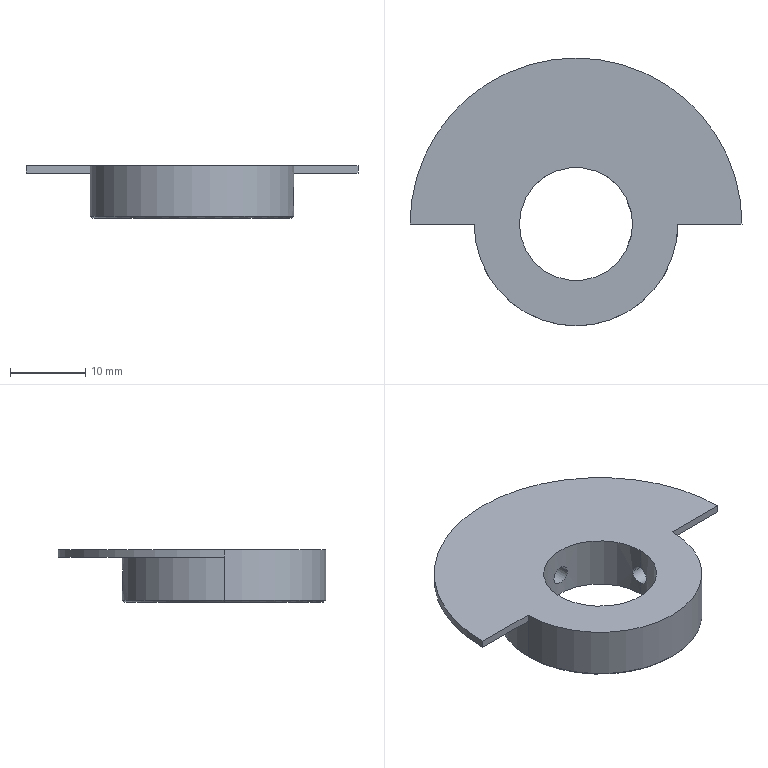Part | NX | 1 solid | 20 faces | box 44 x 35.5 x 7 mm | volume 3181 mm3 | cylinder 9 | plane 5 | spline 4 | cone 2 | commonest cylinder face diameters 2.5 x4 15 x2 27 x2 44 x1
STEP:
#1=CARTESIAN_POINT('',(13.2,0.,-7.));
#2=VERTEX_POINT('',#1);
#3=CARTESIAN_POINT('',(-13.2,0.,-7.));
#4=VERTEX_POINT('',#3);
#5=CARTESIAN_POINT('',(0.,0.,-7.));
#6=DIRECTION('',(0.,0.,-1.));
#7=DIRECTION('',(1.,0.,0.));
#8=AXIS2_PLACEMENT_3D('',#5,#6,#7);
#9=CIRCLE('',#8,13.2);
#10=EDGE_CURVE('',#2,#4,#9,.T.);
#11=ORIENTED_EDGE('',*,*,#10,.T.);
#12=CARTESIAN_POINT('',(0.,0.,-7.));
#13=DIRECTION('',(0.,0.,-1.));
#14=DIRECTION('',(1.,0.,0.));
#15=AXIS2_PLACEMENT_3D('',#12,#13,#14);
#16=CIRCLE('',#15,13.2);
#17=EDGE_CURVE('',#4,#2,#16,.T.);
#18=ORIENTED_EDGE('',*,*,#17,.T.);
#19=EDGE_LOOP('',(#11,#18));
#20=FACE_BOUND('',#19,.T.);
#21=CARTESIAN_POINT('',(7.5,0.,-7.));
#22=VERTEX_POINT('',#21);
#23=CARTESIAN_POINT('',(-7.5,0.,-7.));
#24=VERTEX_POINT('',#23);
#25=CARTESIAN_POINT('',(0.,0.,-7.));
#26=DIRECTION('',(0.,0.,1.));
#27=DIRECTION('',(1.,0.,0.));
#28=AXIS2_PLACEMENT_3D('',#25,#26,#27);
#29=CIRCLE('',#28,7.5);
#30=EDGE_CURVE('',#22,#24,#29,.T.);
#31=ORIENTED_EDGE('',*,*,#30,.T.);
#32=CARTESIAN_POINT('',(0.,0.,-7.));
#33=DIRECTION('',(0.,0.,1.));
#34=DIRECTION('',(1.,0.,0.));
#35=AXIS2_PLACEMENT_3D('',#32,#33,#34);
#36=CIRCLE('',#35,7.5);
#37=EDGE_CURVE('',#24,#22,#36,.T.);
#38=ORIENTED_EDGE('',*,*,#37,.T.);
#39=EDGE_LOOP('',(#31,#38));
#40=FACE_BOUND('',#39,.T.);
#41=CARTESIAN_POINT('',(0.,0.,-7.));
#42=DIRECTION('',(0.,0.,1.));
#43=DIRECTION('',(1.,0.,0.));
#44=AXIS2_PLACEMENT_3D('',#41,#42,#43);
#45=PLANE('',#44);
#46=ADVANCED_FACE('',(#20,#40),#45,.F.);
#47=CARTESIAN_POINT('',(-13.5,0.,0.));
#48=VERTEX_POINT('',#47);
#49=CARTESIAN_POINT('',(-13.5,0.,-1.));
#50=VERTEX_POINT('',#49);
#51=CARTESIAN_POINT('',(-13.5,0.,0.));
#52=DIRECTION('',(0.,0.,-1.));
#53=VECTOR('',#52,1000.);
#54=LINE('',#51,#53);
#55=EDGE_CURVE('',#48,#50,#54,.T.);
#56=ORIENTED_EDGE('',*,*,#55,.T.);
#57=CARTESIAN_POINT('',(-13.5,0.,-6.7));
#58=VERTEX_POINT('',#57);
#59=CARTESIAN_POINT('',(-13.5,0.,0.));
#60=DIRECTION('',(0.,0.,-1.));
#61=VECTOR('',#60,1000.);
#62=LINE('',#59,#61);
#63=EDGE_CURVE('',#58,#50,#62,.F.);
#64=ORIENTED_EDGE('',*,*,#63,.F.);
#65=CARTESIAN_POINT('',(13.5,0.,-6.7));
#66=VERTEX_POINT('',#65);
#67=CARTESIAN_POINT('',(0.,0.,-6.7));
#68=DIRECTION('',(0.,0.,-1.));
#69=DIRECTION('',(1.,0.,0.));
#70=AXIS2_PLACEMENT_3D('',#67,#68,#69);
#71=CIRCLE('',#70,13.5);
#72=EDGE_CURVE('',#66,#58,#71,.T.);
#73=ORIENTED_EDGE('',*,*,#72,.F.);
#74=CARTESIAN_POINT('',(13.5,0.,-5.7));
#75=VERTEX_POINT('',#74);
#76=CARTESIAN_POINT('',(13.5,0.,0.));
#77=DIRECTION('',(0.,0.,-1.));
#78=VECTOR('',#77,1000.);
#79=LINE('',#76,#78);
#80=EDGE_CURVE('',#75,#66,#79,.T.);
#81=ORIENTED_EDGE('',*,*,#80,.F.);
#82=CARTESIAN_POINT('',(13.5,-0.01096,-5.7));
#83=VERTEX_POINT('',#82);
#84=CARTESIAN_POINT('',(13.5,0.,-5.7));
#85=CARTESIAN_POINT('',(13.5,-0.003653,-5.7));
#86=CARTESIAN_POINT('',(13.5,-0.007306,-5.7));
#87=CARTESIAN_POINT('',(13.5,-0.01096,-5.7));
#88=B_SPLINE_CURVE_WITH_KNOTS('',3,(#84,#85,#86,#87),.UNSPECIFIED.,.F.,.F.,(4,4),(0.,1.),.UNSPECIFIED.);
#89=EDGE_CURVE('',#75,#83,#88,.T.);
#90=ORIENTED_EDGE('',*,*,#89,.T.);
#91=CARTESIAN_POINT('',(13.5,0.,-2.3));
#92=VERTEX_POINT('',#91);
#93=CARTESIAN_POINT('',(13.5,-0.01096,-5.7));
#94=CARTESIAN_POINT('',(13.499,-0.9006,-5.694));
#95=CARTESIAN_POINT('',(13.303,-2.364,-3.994));
#96=CARTESIAN_POINT('',(13.5,-0.8891,-2.3));
#97=CARTESIAN_POINT('',(13.5,0.,-2.3));
#98=B_SPLINE_CURVE_WITH_KNOTS('',3,(#93,#94,#95,#96,#97),.UNSPECIFIED.,.F.,.F.,(4,1,4),(0.,0.5,1.),.UNSPECIFIED.);
#99=EDGE_CURVE('',#83,#92,#98,.T.);
#100=ORIENTED_EDGE('',*,*,#99,.T.);
#101=CARTESIAN_POINT('',(13.5,0.,-1.));
#102=VERTEX_POINT('',#101);
#103=CARTESIAN_POINT('',(13.5,0.,0.));
#104=DIRECTION('',(0.,0.,-1.));
#105=VECTOR('',#104,1000.);
#106=LINE('',#103,#105);
#107=EDGE_CURVE('',#92,#102,#106,.F.);
#108=ORIENTED_EDGE('',*,*,#107,.T.);
#109=CARTESIAN_POINT('',(13.5,0.,0.));
#110=VERTEX_POINT('',#109);
#111=CARTESIAN_POINT('',(13.5,0.,0.));
#112=DIRECTION('',(0.,0.,-1.));
#113=VECTOR('',#112,1000.);
#114=LINE('',#111,#113);
#115=EDGE_CURVE('',#110,#102,#114,.T.);
#116=ORIENTED_EDGE('',*,*,#115,.F.);
#117=CARTESIAN_POINT('',(0.,0.,0.));
#118=DIRECTION('',(0.,0.,1.));
#119=DIRECTION('',(-1.,0.,0.));
#120=AXIS2_PLACEMENT_3D('',#117,#118,#119);
#121=CIRCLE('',#120,13.5);
#122=EDGE_CURVE('',#48,#110,#121,.T.);
#123=ORIENTED_EDGE('',*,*,#122,.F.);
#124=EDGE_LOOP('',(#56,#64,#73,#81,#90,#100,#108,#116,#123));
#125=FACE_BOUND('',#124,.T.);
#126=CARTESIAN_POINT('',(0.,0.,0.));
#127=DIRECTION('',(0.,0.,-1.));
#128=DIRECTION('',(-1.,0.,0.));
#129=AXIS2_PLACEMENT_3D('',#126,#127,#128);
#130=CYLINDRICAL_SURFACE('',#129,13.5);
#131=ADVANCED_FACE('',(#125),#130,.T.);
#132=CARTESIAN_POINT('',(0.009525,13.24,-5.25));
#133=VERTEX_POINT('',#132);
#134=CARTESIAN_POINT('',(1.25,13.182,-4.));
#135=VERTEX_POINT('',#134);
#136=CARTESIAN_POINT('',(1.25,13.182,-4.));
#137=CARTESIAN_POINT('',(1.25,13.182,-4.158));
#138=CARTESIAN_POINT('',(1.181,13.188,-4.446));
#139=CARTESIAN_POINT('',(1.074,13.198,-4.653));
#140=CARTESIAN_POINT('',(0.8909,13.211,-4.899));
#141=CARTESIAN_POINT('',(0.6426,13.225,-5.08));
#142=CARTESIAN_POINT('',(0.4451,13.234,-5.18));
#143=CARTESIAN_POINT('',(0.1615,13.24,-5.249));
#144=CARTESIAN_POINT('',(0.009525,13.24,-5.25));
#145=B_SPLINE_CURVE_WITH_KNOTS('',3,(#136,#137,#138,#139,#140,#141,#142,#143,#144),.UNSPECIFIED.,.F.,.F.,(4,1,1,1,1,1,4),(0.,0.25,0.375,0.5,0.625,0.75,1.),.UNSPECIFIED.);
#146=EDGE_CURVE('',#133,#135,#145,.F.);
#147=ORIENTED_EDGE('',*,*,#146,.T.);
#148=CARTESIAN_POINT('',(-0.009148,13.24,-2.75));
#149=VERTEX_POINT('',#148);
#150=CARTESIAN_POINT('',(-0.009147,13.24,-2.75));
#151=CARTESIAN_POINT('',(0.1457,13.24,-2.749));
#152=CARTESIAN_POINT('',(0.4278,13.234,-2.813));
#153=CARTESIAN_POINT('',(0.6331,13.225,-2.915));
#154=CARTESIAN_POINT('',(0.8826,13.212,-3.093));
#155=CARTESIAN_POINT('',(1.072,13.198,-3.344));
#156=CARTESIAN_POINT('',(1.178,13.189,-3.548));
#157=CARTESIAN_POINT('',(1.25,13.182,-3.841));
#158=CARTESIAN_POINT('',(1.25,13.182,-4.));
#159=B_SPLINE_CURVE_WITH_KNOTS('',3,(#150,#151,#152,#153,#154,#155,#156,#157,#158),.UNSPECIFIED.,.F.,.F.,(4,1,1,1,1,1,4),(0.,0.25,0.375,0.5,0.625,0.75,1.),.UNSPECIFIED.);
#160=EDGE_CURVE('',#135,#149,#159,.F.);
#161=ORIENTED_EDGE('',*,*,#160,.T.);
#162=CARTESIAN_POINT('',(-0.01305,13.5,-2.3));
#163=VERTEX_POINT('',#162);
#164=CARTESIAN_POINT('',(-0.009148,13.24,-2.75));
#165=CARTESIAN_POINT('',(-0.01305,13.5,-2.3));
#166=B_SPLINE_CURVE_WITH_KNOTS('',1,(#164,#165),.UNSPECIFIED.,.F.,.F.,(2,2),(0.,1.),.UNSPECIFIED.);
#167=EDGE_CURVE('',#163,#149,#166,.F.);
#168=ORIENTED_EDGE('',*,*,#167,.F.);
#169=CARTESIAN_POINT('',(0.01314,13.5,-5.7));
#170=VERTEX_POINT('',#169);
#171=CARTESIAN_POINT('',(0.01314,13.5,-5.7));
#172=CARTESIAN_POINT('',(0.9097,13.499,-5.692));
#173=CARTESIAN_POINT('',(2.362,13.303,-3.98));
#174=CARTESIAN_POINT('',(0.8851,13.501,-2.294));
#175=CARTESIAN_POINT('',(-0.01305,13.5,-2.3));
#176=B_SPLINE_CURVE_WITH_KNOTS('',3,(#171,#172,#173,#174,#175),.UNSPECIFIED.,.F.,.F.,(4,1,4),(0.,0.5,1.),.UNSPECIFIED.);
#177=EDGE_CURVE('',#170,#163,#176,.T.);
#178=ORIENTED_EDGE('',*,*,#177,.F.);
#179=CARTESIAN_POINT('',(0.009525,13.24,-5.25));
#180=CARTESIAN_POINT('',(0.01314,13.5,-5.7));
#181=B_SPLINE_CURVE_WITH_KNOTS('',1,(#179,#180),.UNSPECIFIED.,.F.,.F.,(2,2),(0.,1.),.UNSPECIFIED.);
#182=EDGE_CURVE('',#170,#133,#181,.F.);
#183=ORIENTED_EDGE('',*,*,#182,.T.);
#184=EDGE_LOOP('',(#147,#161,#168,#178,#183));
#185=FACE_BOUND('',#184,.T.);
#186=CARTESIAN_POINT('',(0.009525,13.24,-5.25));
#187=CARTESIAN_POINT('',(0.01314,13.5,-5.7));
#188=CARTESIAN_POINT('',(0.01524,13.24,-5.25));
#189=CARTESIAN_POINT('',(0.02103,13.5,-5.7));
#190=CARTESIAN_POINT('',(0.02096,13.24,-5.25));
#191=CARTESIAN_POINT('',(0.02892,13.5,-5.7));
#192=CARTESIAN_POINT('',(0.05049,13.24,-5.249));
#193=CARTESIAN_POINT('',(0.06965,13.5,-5.699));
#194=CARTESIAN_POINT('',(0.07427,13.24,-5.248));
#195=CARTESIAN_POINT('',(0.1025,13.5,-5.697));
#196=CARTESIAN_POINT('',(0.1973,13.239,-5.238));
#197=CARTESIAN_POINT('',(0.2718,13.498,-5.682));
#198=CARTESIAN_POINT('',(0.295,13.237,-5.219));
#199=CARTESIAN_POINT('',(0.4066,13.494,-5.652));
#200=CARTESIAN_POINT('',(0.586,13.229,-5.123));
#201=CARTESIAN_POINT('',(0.7985,13.479,-5.509));
#202=CARTESIAN_POINT('',(0.7633,13.219,-5.012));
#203=CARTESIAN_POINT('',(1.031,13.462,-5.344));
#204=CARTESIAN_POINT('',(1.05,13.2,-4.71));
#205=CARTESIAN_POINT('',(1.391,13.429,-4.925));
#206=CARTESIAN_POINT('',(1.154,13.191,-4.524));
#207=CARTESIAN_POINT('',(1.516,13.415,-4.679));
#208=CARTESIAN_POINT('',(1.262,13.181,-4.118));
#209=CARTESIAN_POINT('',(1.644,13.4,-4.15));
#210=CARTESIAN_POINT('',(1.264,13.181,-3.902));
#211=CARTESIAN_POINT('',(1.646,13.399,-3.876));
#212=CARTESIAN_POINT('',(1.162,13.19,-3.492));
#213=CARTESIAN_POINT('',(1.525,13.414,-3.342));
#214=CARTESIAN_POINT('',(1.058,13.199,-3.303));
#215=CARTESIAN_POINT('',(1.402,13.428,-3.092));
#216=CARTESIAN_POINT('',(0.7739,13.218,-2.996));
#217=CARTESIAN_POINT('',(1.044,13.461,-2.668));
#218=CARTESIAN_POINT('',(0.5977,13.228,-2.883));
#219=CARTESIAN_POINT('',(0.8144,13.478,-2.501));
#220=CARTESIAN_POINT('',(0.269,13.238,-2.771));
#221=CARTESIAN_POINT('',(0.3717,13.496,-2.333));
#222=CARTESIAN_POINT('',(0.1303,13.24,-2.749));
#223=CARTESIAN_POINT('',(0.1794,13.5,-2.299));
#224=CARTESIAN_POINT('',(-0.009148,13.24,-2.75));
#225=CARTESIAN_POINT('',(-0.01305,13.5,-2.3));
#226=B_SPLINE_SURFACE_WITH_KNOTS('',3,1,((#186,#187),(#188,#189),(#190,#191),(#192,#193),(#194,#195),(#196,#197),(#198,#199),(#200,#201),(#202,#203),(#204,#205),(#206,#207),(#208,#209),(#210,#211),(#212,#213),(#214,#215),(#216,#217),(#218,#219),(#220,#221),(#222,#223),(#224,#225)),.RULED_SURF.,.F.,.F.,.F.,(4,2,2,2,2,2,2,2,2,4),(2,2),(0.,0.02041,0.1054,0.4606,1.192,1.919,2.647,3.381,4.112,4.613),(0.,1.),.UNSPECIFIED.);
#227=ADVANCED_FACE('',(#185),#226,.T.);
#228=CARTESIAN_POINT('',(-22.,0.,-1.));
#229=VERTEX_POINT('',#228);
#230=CARTESIAN_POINT('',(-13.5,0.,-1.));
#231=DIRECTION('',(-1.,0.,0.));
#232=VECTOR('',#231,1000.);
#233=LINE('',#230,#232);
#234=EDGE_CURVE('',#50,#229,#233,.T.);
#235=ORIENTED_EDGE('',*,*,#234,.T.);
#236=CARTESIAN_POINT('',(22.,0.,-1.));
#237=VERTEX_POINT('',#236);
#238=CARTESIAN_POINT('',(0.,0.,-1.));
#239=DIRECTION('',(0.,0.,-1.));
#240=DIRECTION('',(-1.,0.,0.));
#241=AXIS2_PLACEMENT_3D('',#238,#239,#240);
#242=CIRCLE('',#241,22.);
#243=EDGE_CURVE('',#229,#237,#242,.T.);
#244=ORIENTED_EDGE('',*,*,#243,.T.);
#245=CARTESIAN_POINT('',(22.,0.,-1.));
#246=DIRECTION('',(-1.,0.,0.));
#247=VECTOR('',#246,1000.);
#248=LINE('',#245,#247);
#249=EDGE_CURVE('',#237,#102,#248,.T.);
#250=ORIENTED_EDGE('',*,*,#249,.T.);
#251=CARTESIAN_POINT('',(0.,0.,-1.));
#252=DIRECTION('',(0.,0.,1.));
#253=DIRECTION('',(-1.,0.,0.));
#254=AXIS2_PLACEMENT_3D('',#251,#252,#253);
#255=CIRCLE('',#254,13.5);
#256=EDGE_CURVE('',#102,#50,#255,.T.);
#257=ORIENTED_EDGE('',*,*,#256,.T.);
#258=EDGE_LOOP('',(#235,#244,#250,#257));
#259=FACE_BOUND('',#258,.T.);
#260=CARTESIAN_POINT('',(0.,0.,-1.));
#261=DIRECTION('',(0.,0.,1.));
#262=DIRECTION('',(1.,0.,0.));
#263=AXIS2_PLACEMENT_3D('',#260,#261,#262);
#264=PLANE('',#263);
#265=ADVANCED_FACE('',(#259),#264,.F.);
#266=CARTESIAN_POINT('',(-22.,0.,0.));
#267=VERTEX_POINT('',#266);
#268=CARTESIAN_POINT('',(0.,0.,0.));
#269=DIRECTION('',(-1.,0.,0.));
#270=VECTOR('',#269,1000.);
#271=LINE('',#268,#270);
#272=EDGE_CURVE('',#48,#267,#271,.T.);
#273=ORIENTED_EDGE('',*,*,#272,.T.);
#274=CARTESIAN_POINT('',(-22.,0.,0.));
#275=DIRECTION('',(0.,0.,-1.));
#276=VECTOR('',#275,1000.);
#277=LINE('',#274,#276);
#278=EDGE_CURVE('',#267,#229,#277,.T.);
#279=ORIENTED_EDGE('',*,*,#278,.T.);
#280=ORIENTED_EDGE('',*,*,#234,.F.);
#281=ORIENTED_EDGE('',*,*,#55,.F.);
#282=EDGE_LOOP('',(#273,#279,#280,#281));
#283=FACE_BOUND('',#282,.T.);
#284=CARTESIAN_POINT('',(-22.,0.,0.));
#285=DIRECTION('',(0.,1.,0.));
#286=DIRECTION('',(1.,0.,0.));
#287=AXIS2_PLACEMENT_3D('',#284,#285,#286);
#288=PLANE('',#287);
#289=ADVANCED_FACE('',(#283),#288,.F.);
#290=CARTESIAN_POINT('',(22.,0.,0.));
#291=VERTEX_POINT('',#290);
#292=CARTESIAN_POINT('',(0.,0.,0.));
#293=DIRECTION('',(-1.,0.,0.));
#294=VECTOR('',#293,1000.);
#295=LINE('',#292,#294);
#296=EDGE_CURVE('',#291,#110,#295,.T.);
#297=ORIENTED_EDGE('',*,*,#296,.F.);
#298=CARTESIAN_POINT('',(0.,0.,0.));
#299=DIRECTION('',(0.,0.,1.));
#300=DIRECTION('',(-1.,0.,0.));
#301=AXIS2_PLACEMENT_3D('',#298,#299,#300);
#302=CIRCLE('',#301,22.);
#303=EDGE_CURVE('',#291,#267,#302,.T.);
#304=ORIENTED_EDGE('',*,*,#303,.T.);
#305=ORIENTED_EDGE('',*,*,#272,.F.);
#306=ORIENTED_EDGE('',*,*,#122,.T.);
#307=EDGE_LOOP('',(#297,#304,#305,#306));
#308=FACE_BOUND('',#307,.T.);
#309=CARTESIAN_POINT('',(7.5,0.,0.));
#310=VERTEX_POINT('',#309);
#311=CARTESIAN_POINT('',(-7.5,0.,0.));
#312=VERTEX_POINT('',#311);
#313=CARTESIAN_POINT('',(0.,0.,0.));
#314=DIRECTION('',(0.,0.,1.));
#315=DIRECTION('',(1.,0.,0.));
#316=AXIS2_PLACEMENT_3D('',#313,#314,#315);
#317=CIRCLE('',#316,7.5);
#318=EDGE_CURVE('',#310,#312,#317,.T.);
#319=ORIENTED_EDGE('',*,*,#318,.F.);
#320=CARTESIAN_POINT('',(0.,0.,0.));
#321=DIRECTION('',(0.,0.,1.));
#322=DIRECTION('',(1.,0.,0.));
#323=AXIS2_PLACEMENT_3D('',#320,#321,#322);
#324=CIRCLE('',#323,7.5);
#325=EDGE_CURVE('',#312,#310,#324,.T.);
#326=ORIENTED_EDGE('',*,*,#325,.F.);
#327=EDGE_LOOP('',(#319,#326));
#328=FACE_BOUND('',#327,.T.);
#329=CARTESIAN_POINT('',(0.,0.,0.));
#330=DIRECTION('',(0.,0.,1.));
#331=DIRECTION('',(1.,0.,0.));
#332=AXIS2_PLACEMENT_3D('',#329,#330,#331);
#333=PLANE('',#332);
#334=ADVANCED_FACE('',(#308,#328),#333,.T.);
#335=ORIENTED_EDGE('',*,*,#30,.F.);
#336=CARTESIAN_POINT('',(7.5,0.,-5.25));
#337=VERTEX_POINT('',#336);
#338=CARTESIAN_POINT('',(7.5,0.,0.));
#339=DIRECTION('',(0.,0.,-1.));
#340=VECTOR('',#339,1000.);
#341=LINE('',#338,#340);
#342=EDGE_CURVE('',#22,#337,#341,.F.);
#343=ORIENTED_EDGE('',*,*,#342,.T.);
#344=CARTESIAN_POINT('',(7.395,1.25,-4.));
#345=VERTEX_POINT('',#344);
#346=CARTESIAN_POINT('',(7.5,0.,-5.25));
#347=CARTESIAN_POINT('',(7.5,0.6634,-5.25));
#348=CARTESIAN_POINT('',(7.395,1.25,-4.664));
#349=CARTESIAN_POINT('',(7.395,1.25,-4.));
#350=B_SPLINE_CURVE_WITH_KNOTS('',3,(#346,#347,#348,#349),.UNSPECIFIED.,.F.,.F.,(4,4),(0.,1.),.UNSPECIFIED.);
#351=EDGE_CURVE('',#345,#337,#350,.F.);
#352=ORIENTED_EDGE('',*,*,#351,.F.);
#353=CARTESIAN_POINT('',(7.5,0.,-2.75));
#354=VERTEX_POINT('',#353);
#355=CARTESIAN_POINT('',(7.395,1.25,-4.));
#356=CARTESIAN_POINT('',(7.395,1.25,-3.336));
#357=CARTESIAN_POINT('',(7.5,0.6635,-2.75));
#358=CARTESIAN_POINT('',(7.5,0.,-2.75));
#359=B_SPLINE_CURVE_WITH_KNOTS('',3,(#355,#356,#357,#358),.UNSPECIFIED.,.F.,.F.,(4,4),(0.,1.),.UNSPECIFIED.);
#360=EDGE_CURVE('',#354,#345,#359,.F.);
#361=ORIENTED_EDGE('',*,*,#360,.F.);
#362=CARTESIAN_POINT('',(7.5,0.,0.));
#363=DIRECTION('',(0.,0.,-1.));
#364=VECTOR('',#363,1000.);
#365=LINE('',#362,#364);
#366=EDGE_CURVE('',#310,#354,#365,.T.);
#367=ORIENTED_EDGE('',*,*,#366,.F.);
#368=ORIENTED_EDGE('',*,*,#318,.T.);
#369=CARTESIAN_POINT('',(-7.5,0.,0.));
#370=DIRECTION('',(0.,0.,-1.));
#371=VECTOR('',#370,1000.);
#372=LINE('',#369,#371);
#373=EDGE_CURVE('',#24,#312,#372,.F.);
#374=ORIENTED_EDGE('',*,*,#373,.F.);
#375=EDGE_LOOP('',(#335,#343,#352,#361,#367,#368,#374));
#376=FACE_BOUND('',#375,.T.);
#377=CARTESIAN_POINT('',(1.25,7.395,-4.));
#378=VERTEX_POINT('',#377);
#379=CARTESIAN_POINT('',(-1.25,7.395,-4.));
#380=VERTEX_POINT('',#379);
#381=CARTESIAN_POINT('',(-1.25,7.395,-4.));
#382=CARTESIAN_POINT('',(-1.25,7.395,-3.668));
#383=CARTESIAN_POINT('',(-0.9802,7.448,-3.024));
#384=CARTESIAN_POINT('',(0.0002674,7.526,-2.613));
#385=CARTESIAN_POINT('',(0.9792,7.448,-3.023));
#386=CARTESIAN_POINT('',(1.25,7.395,-3.668));
#387=CARTESIAN_POINT('',(1.25,7.395,-4.));
#388=B_SPLINE_CURVE_WITH_KNOTS('',3,(#381,#382,#383,#384,#385,#386,#387),.UNSPECIFIED.,.F.,.F.,(4,1,1,1,4),(0.,0.25,0.5,0.75,1.),.UNSPECIFIED.);
#389=EDGE_CURVE('',#378,#380,#388,.F.);
#390=ORIENTED_EDGE('',*,*,#389,.F.);
#391=CARTESIAN_POINT('',(1.25,7.395,-4.));
#392=CARTESIAN_POINT('',(1.25,7.395,-4.332));
#393=CARTESIAN_POINT('',(0.9795,7.448,-4.977));
#394=CARTESIAN_POINT('',(-0.00005471,7.526,-5.386));
#395=CARTESIAN_POINT('',(-0.9793,7.448,-4.977));
#396=CARTESIAN_POINT('',(-1.25,7.395,-4.332));
#397=CARTESIAN_POINT('',(-1.25,7.395,-4.));
#398=B_SPLINE_CURVE_WITH_KNOTS('',3,(#391,#392,#393,#394,#395,#396,#397),.UNSPECIFIED.,.F.,.F.,(4,1,1,1,4),(0.,0.25,0.5,0.75,1.),.UNSPECIFIED.);
#399=EDGE_CURVE('',#380,#378,#398,.F.);
#400=ORIENTED_EDGE('',*,*,#399,.F.);
#401=EDGE_LOOP('',(#390,#400));
#402=FACE_BOUND('',#401,.T.);
#403=CARTESIAN_POINT('',(0.,0.,0.));
#404=DIRECTION('',(0.,0.,-1.));
#405=DIRECTION('',(1.,0.,0.));
#406=AXIS2_PLACEMENT_3D('',#403,#404,#405);
#407=CYLINDRICAL_SURFACE('',#406,7.5);
#408=ADVANCED_FACE('',(#376,#402),#407,.F.);
#409=ORIENTED_EDGE('',*,*,#249,.F.);
#410=CARTESIAN_POINT('',(22.,0.,0.));
#411=DIRECTION('',(0.,0.,-1.));
#412=VECTOR('',#411,1000.);
#413=LINE('',#410,#412);
#414=EDGE_CURVE('',#291,#237,#413,.T.);
#415=ORIENTED_EDGE('',*,*,#414,.F.);
#416=ORIENTED_EDGE('',*,*,#296,.T.);
#417=ORIENTED_EDGE('',*,*,#115,.T.);
#418=EDGE_LOOP('',(#409,#415,#416,#417));
#419=FACE_BOUND('',#418,.T.);
#420=CARTESIAN_POINT('',(13.5,0.,0.));
#421=DIRECTION('',(0.,1.,0.));
#422=DIRECTION('',(1.,0.,0.));
#423=AXIS2_PLACEMENT_3D('',#420,#421,#422);
#424=PLANE('',#423);
#425=ADVANCED_FACE('',(#419),#424,.F.);
#426=ORIENTED_EDGE('',*,*,#414,.T.);
#427=ORIENTED_EDGE('',*,*,#243,.F.);
#428=ORIENTED_EDGE('',*,*,#278,.F.);
#429=ORIENTED_EDGE('',*,*,#303,.F.);
#430=EDGE_LOOP('',(#426,#427,#428,#429));
#431=FACE_BOUND('',#430,.T.);
#432=CARTESIAN_POINT('',(0.,0.,0.));
#433=DIRECTION('',(0.,0.,-1.));
#434=DIRECTION('',(-1.,0.,0.));
#435=AXIS2_PLACEMENT_3D('',#432,#433,#434);
#436=CYLINDRICAL_SURFACE('',#435,22.);
#437=ADVANCED_FACE('',(#431),#436,.T.);
#438=ORIENTED_EDGE('',*,*,#389,.T.);
#439=CARTESIAN_POINT('',(-1.25,13.182,-4.));
#440=VERTEX_POINT('',#439);
#441=CARTESIAN_POINT('',(-1.25,13.5,-4.));
#442=DIRECTION('',(0.,1.,0.));
#443=VECTOR('',#442,1000.);
#444=LINE('',#441,#443);
#445=EDGE_CURVE('',#440,#380,#444,.F.);
#446=ORIENTED_EDGE('',*,*,#445,.F.);
#447=CARTESIAN_POINT('',(-1.25,13.182,-4.));
#448=CARTESIAN_POINT('',(-1.25,13.182,-3.842));
#449=CARTESIAN_POINT('',(-1.179,13.188,-3.551));
#450=CARTESIAN_POINT('',(-1.076,13.197,-3.351));
#451=CARTESIAN_POINT('',(-0.89,13.211,-3.1));
#452=CARTESIAN_POINT('',(-0.6429,13.225,-2.921));
#453=CARTESIAN_POINT('',(-0.4429,13.234,-2.818));
#454=CARTESIAN_POINT('',(-0.1597,13.24,-2.751));
#455=CARTESIAN_POINT('',(-0.009147,13.24,-2.75));
#456=B_SPLINE_CURVE_WITH_KNOTS('',3,(#447,#448,#449,#450,#451,#452,#453,#454,#455),.UNSPECIFIED.,.F.,.F.,(4,1,1,1,1,1,4),(0.,0.25,0.375,0.5,0.625,0.75,1.),.UNSPECIFIED.);
#457=EDGE_CURVE('',#149,#440,#456,.F.);
#458=ORIENTED_EDGE('',*,*,#457,.F.);
#459=ORIENTED_EDGE('',*,*,#160,.F.);
#460=CARTESIAN_POINT('',(1.25,13.5,-4.));
#461=DIRECTION('',(0.,1.,0.));
#462=VECTOR('',#461,1000.);
#463=LINE('',#460,#462);
#464=EDGE_CURVE('',#135,#378,#463,.F.);
#465=ORIENTED_EDGE('',*,*,#464,.T.);
#466=EDGE_LOOP('',(#438,#446,#458,#459,#465));
#467=FACE_BOUND('',#466,.T.);
#468=CARTESIAN_POINT('',(0.,13.5,-4.));
#469=DIRECTION('',(0.,1.,0.));
#470=DIRECTION('',(1.,0.,0.));
#471=AXIS2_PLACEMENT_3D('',#468,#469,#470);
#472=CYLINDRICAL_SURFACE('',#471,1.25);
#473=ADVANCED_FACE('',(#467),#472,.F.);
#474=CARTESIAN_POINT('',(13.182,1.25,-4.));
#475=VERTEX_POINT('',#474);
#476=CARTESIAN_POINT('',(13.24,-0.007631,-5.25));
#477=VERTEX_POINT('',#476);
#478=CARTESIAN_POINT('',(13.24,-0.00763,-5.25));
#479=CARTESIAN_POINT('',(13.24,0.1471,-5.251));
#480=CARTESIAN_POINT('',(13.234,0.4291,-5.187));
#481=CARTESIAN_POINT('',(13.225,0.6337,-5.085));
#482=CARTESIAN_POINT('',(13.212,0.8832,-4.907));
#483=CARTESIAN_POINT('',(13.198,1.072,-4.656));
#484=CARTESIAN_POINT('',(13.189,1.179,-4.452));
#485=CARTESIAN_POINT('',(13.182,1.25,-4.159));
#486=CARTESIAN_POINT('',(13.182,1.25,-4.));
#487=B_SPLINE_CURVE_WITH_KNOTS('',3,(#478,#479,#480,#481,#482,#483,#484,#485,#486),.UNSPECIFIED.,.F.,.F.,(4,1,1,1,1,1,4),(0.,0.25,0.375,0.5,0.625,0.75,1.),.UNSPECIFIED.);
#488=EDGE_CURVE('',#475,#477,#487,.F.);
#489=ORIENTED_EDGE('',*,*,#488,.F.);
#490=CARTESIAN_POINT('',(13.5,1.25,-4.));
#491=DIRECTION('',(1.,0.,0.));
#492=VECTOR('',#491,1000.);
#493=LINE('',#490,#492);
#494=EDGE_CURVE('',#345,#475,#493,.T.);
#495=ORIENTED_EDGE('',*,*,#494,.F.);
#496=ORIENTED_EDGE('',*,*,#351,.T.);
#497=CARTESIAN_POINT('',(7.395,-1.25,-4.));
#498=VERTEX_POINT('',#497);
#499=CARTESIAN_POINT('',(7.5,0.,-5.25));
#500=CARTESIAN_POINT('',(7.5,-0.1196,-5.25));
#501=CARTESIAN_POINT('',(7.493,-0.4003,-5.221));
#502=CARTESIAN_POINT('',(7.448,-0.92,-4.921));
#503=CARTESIAN_POINT('',(7.403,-1.223,-4.397));
#504=CARTESIAN_POINT('',(7.395,-1.25,-4.118));
#505=CARTESIAN_POINT('',(7.395,-1.25,-4.));
#506=B_SPLINE_CURVE_WITH_KNOTS('',3,(#499,#500,#501,#502,#503,#504,#505),.UNSPECIFIED.,.F.,.F.,(4,1,1,1,4),(0.,0.25,0.5,0.75,1.),.UNSPECIFIED.);
#507=EDGE_CURVE('',#337,#498,#506,.T.);
#508=ORIENTED_EDGE('',*,*,#507,.T.);
#509=CARTESIAN_POINT('',(13.182,-1.25,-4.));
#510=VERTEX_POINT('',#509);
#511=CARTESIAN_POINT('',(13.5,-1.25,-4.));
#512=DIRECTION('',(1.,0.,0.));
#513=VECTOR('',#512,1000.);
#514=LINE('',#511,#513);
#515=EDGE_CURVE('',#498,#510,#514,.T.);
#516=ORIENTED_EDGE('',*,*,#515,.T.);
#517=CARTESIAN_POINT('',(13.182,-1.25,-4.));
#518=CARTESIAN_POINT('',(13.182,-1.25,-4.158));
#519=CARTESIAN_POINT('',(13.188,-1.179,-4.449));
#520=CARTESIAN_POINT('',(13.197,-1.076,-4.649));
#521=CARTESIAN_POINT('',(13.211,-0.8894,-4.9));
#522=CARTESIAN_POINT('',(13.225,-0.6423,-5.08));
#523=CARTESIAN_POINT('',(13.234,-0.4417,-5.182));
#524=CARTESIAN_POINT('',(13.24,-0.1583,-5.249));
#525=CARTESIAN_POINT('',(13.24,-0.00763,-5.25));
#526=B_SPLINE_CURVE_WITH_KNOTS('',3,(#517,#518,#519,#520,#521,#522,#523,#524,#525),.UNSPECIFIED.,.F.,.F.,(4,1,1,1,1,1,4),(0.,0.25,0.375,0.5,0.625,0.75,1.),.UNSPECIFIED.);
#527=EDGE_CURVE('',#477,#510,#526,.F.);
#528=ORIENTED_EDGE('',*,*,#527,.F.);
#529=EDGE_LOOP('',(#489,#495,#496,#508,#516,#528));
#530=FACE_BOUND('',#529,.T.);
#531=CARTESIAN_POINT('',(13.5,0.,-4.));
#532=DIRECTION('',(1.,0.,0.));
#533=DIRECTION('',(0.,-1.,0.));
#534=AXIS2_PLACEMENT_3D('',#531,#532,#533);
#535=CYLINDRICAL_SURFACE('',#534,1.25);
#536=ADVANCED_FACE('',(#530),#535,.F.);
#537=ORIENTED_EDGE('',*,*,#488,.T.);
#538=CARTESIAN_POINT('',(13.24,-0.007631,-5.25));
#539=CARTESIAN_POINT('',(13.5,-0.01096,-5.7));
#540=B_SPLINE_CURVE_WITH_KNOTS('',1,(#538,#539),.UNSPECIFIED.,.F.,.F.,(2,2),(0.,1.),.UNSPECIFIED.);
#541=EDGE_CURVE('',#83,#477,#540,.F.);
#542=ORIENTED_EDGE('',*,*,#541,.F.);
#543=ORIENTED_EDGE('',*,*,#89,.F.);
#544=CARTESIAN_POINT('',(13.5,0.01105,-2.3));
#545=VERTEX_POINT('',#544);
#546=CARTESIAN_POINT('',(13.5,0.01105,-2.3));
#547=CARTESIAN_POINT('',(13.499,0.9058,-2.306));
#548=CARTESIAN_POINT('',(13.303,2.358,-4.01));
#549=CARTESIAN_POINT('',(13.5,0.896,-5.699));
#550=CARTESIAN_POINT('',(13.5,0.,-5.7));
#551=B_SPLINE_CURVE_WITH_KNOTS('',3,(#546,#547,#548,#549,#550),.UNSPECIFIED.,.F.,.F.,(4,1,4),(0.,0.5,1.),.UNSPECIFIED.);
#552=EDGE_CURVE('',#545,#75,#551,.T.);
#553=ORIENTED_EDGE('',*,*,#552,.F.);
#554=CARTESIAN_POINT('',(13.24,0.008007,-2.75));
#555=VERTEX_POINT('',#554);
#556=CARTESIAN_POINT('',(13.24,0.008007,-2.75));
#557=CARTESIAN_POINT('',(13.5,0.01105,-2.3));
#558=B_SPLINE_CURVE_WITH_KNOTS('',1,(#556,#557),.UNSPECIFIED.,.F.,.F.,(2,2),(0.,1.),.UNSPECIFIED.);
#559=EDGE_CURVE('',#545,#555,#558,.F.);
#560=ORIENTED_EDGE('',*,*,#559,.T.);
#561=CARTESIAN_POINT('',(13.182,1.25,-4.));
#562=CARTESIAN_POINT('',(13.182,1.25,-3.842));
#563=CARTESIAN_POINT('',(13.188,1.181,-3.553));
#564=CARTESIAN_POINT('',(13.198,1.074,-3.347));
#565=CARTESIAN_POINT('',(13.211,0.8903,-3.101));
#566=CARTESIAN_POINT('',(13.225,0.642,-2.92));
#567=CARTESIAN_POINT('',(13.234,0.4439,-2.819));
#568=CARTESIAN_POINT('',(13.24,0.1601,-2.751));
#569=CARTESIAN_POINT('',(13.24,0.008007,-2.75));
#570=B_SPLINE_CURVE_WITH_KNOTS('',3,(#561,#562,#563,#564,#565,#566,#567,#568,#569),.UNSPECIFIED.,.F.,.F.,(4,1,1,1,1,1,4),(0.,0.25,0.375,0.5,0.625,0.75,1.),.UNSPECIFIED.);
#571=EDGE_CURVE('',#555,#475,#570,.F.);
#572=ORIENTED_EDGE('',*,*,#571,.T.);
#573=EDGE_LOOP('',(#537,#542,#543,#553,#560,#572));
#574=FACE_BOUND('',#573,.T.);
#575=CARTESIAN_POINT('',(13.24,0.008007,-2.75));
#576=CARTESIAN_POINT('',(13.5,0.01105,-2.3));
#577=CARTESIAN_POINT('',(13.24,0.01372,-2.75));
#578=CARTESIAN_POINT('',(13.5,0.01893,-2.3));
#579=CARTESIAN_POINT('',(13.24,0.01944,-2.75));
#580=CARTESIAN_POINT('',(13.5,0.02682,-2.3));
#581=CARTESIAN_POINT('',(13.24,0.04897,-2.751));
#582=CARTESIAN_POINT('',(13.5,0.06756,-2.301));
#583=CARTESIAN_POINT('',(13.24,0.07275,-2.752));
#584=CARTESIAN_POINT('',(13.5,0.1004,-2.303));
#585=CARTESIAN_POINT('',(13.239,0.1958,-2.761));
#586=CARTESIAN_POINT('',(13.498,0.2697,-2.318));
#587=CARTESIAN_POINT('',(13.237,0.2935,-2.781));
#588=CARTESIAN_POINT('',(13.495,0.4045,-2.348));
#589=CARTESIAN_POINT('',(13.229,0.5846,-2.876));
#590=CARTESIAN_POINT('',(13.479,0.7967,-2.49));
#591=CARTESIAN_POINT('',(13.219,0.7622,-2.987));
#592=CARTESIAN_POINT('',(13.462,1.029,-2.655));
#593=CARTESIAN_POINT('',(13.2,1.049,-3.289));
#594=CARTESIAN_POINT('',(13.429,1.39,-3.073));
#595=CARTESIAN_POINT('',(13.191,1.154,-3.475));
#596=CARTESIAN_POINT('',(13.415,1.515,-3.319));
#597=CARTESIAN_POINT('',(13.181,1.262,-3.881));
#598=CARTESIAN_POINT('',(13.4,1.644,-3.849));
#599=CARTESIAN_POINT('',(13.181,1.264,-4.097));
#600=CARTESIAN_POINT('',(13.399,1.646,-4.123));
#601=CARTESIAN_POINT('',(13.19,1.162,-4.507));
#602=CARTESIAN_POINT('',(13.414,1.525,-4.657));
#603=CARTESIAN_POINT('',(13.199,1.059,-4.697));
#604=CARTESIAN_POINT('',(13.428,1.402,-4.908));
#605=CARTESIAN_POINT('',(13.218,0.7742,-5.003));
#606=CARTESIAN_POINT('',(13.461,1.045,-5.332));
#607=CARTESIAN_POINT('',(13.228,0.598,-5.117));
#608=CARTESIAN_POINT('',(13.478,0.8148,-5.499));
#609=CARTESIAN_POINT('',(13.238,0.2698,-5.229));
#610=CARTESIAN_POINT('',(13.496,0.3728,-5.667));
#611=CARTESIAN_POINT('',(13.24,0.1314,-5.251));
#612=CARTESIAN_POINT('',(13.5,0.181,-5.701));
#613=CARTESIAN_POINT('',(13.24,-0.007631,-5.25));
#614=CARTESIAN_POINT('',(13.5,-0.01096,-5.7));
#615=B_SPLINE_SURFACE_WITH_KNOTS('',3,1,((#575,#576),(#577,#578),(#579,#580),(#581,#582),(#583,#584),(#585,#586),(#587,#588),(#589,#590),(#591,#592),(#593,#594),(#595,#596),(#597,#598),(#599,#600),(#601,#602),(#603,#604),(#605,#606),(#607,#608),(#609,#610),(#611,#612),(#613,#614)),.RULED_SURF.,.F.,.F.,.F.,(4,2,2,2,2,2,2,2,2,4),(2,2),(0.,0.02041,0.1054,0.4605,1.193,1.92,2.648,3.383,4.114,4.613),(0.,1.),.UNSPECIFIED.);
#616=ADVANCED_FACE('',(#574),#615,.T.);
#617=CARTESIAN_POINT('',(0.,0.,-6.7));
#618=DIRECTION('',(0.,0.,-1.));
#619=DIRECTION('',(1.,0.,0.));
#620=AXIS2_PLACEMENT_3D('',#617,#618,#619);
#621=CIRCLE('',#620,13.5);
#622=EDGE_CURVE('',#58,#66,#621,.T.);
#623=ORIENTED_EDGE('',*,*,#622,.T.);
#624=CARTESIAN_POINT('',(13.5,0.,-6.7));
#625=DIRECTION('',(0.7071,0.,0.7071));
#626=VECTOR('',#625,1000.);
#627=LINE('',#624,#626);
#628=EDGE_CURVE('',#2,#66,#627,.T.);
#629=ORIENTED_EDGE('',*,*,#628,.F.);
#630=ORIENTED_EDGE('',*,*,#17,.F.);
#631=CARTESIAN_POINT('',(-13.5,0.,-6.7));
#632=DIRECTION('',(-0.7071,0.,0.7071));
#633=VECTOR('',#632,1000.);
#634=LINE('',#631,#633);
#635=EDGE_CURVE('',#4,#58,#634,.T.);
#636=ORIENTED_EDGE('',*,*,#635,.T.);
#637=EDGE_LOOP('',(#623,#629,#630,#636));
#638=FACE_BOUND('',#637,.T.);
#639=CARTESIAN_POINT('',(0.,0.,-6.7));
#640=DIRECTION('',(0.,0.,1.));
#641=DIRECTION('',(1.,0.,0.));
#642=AXIS2_PLACEMENT_3D('',#639,#640,#641);
#643=CONICAL_SURFACE('',#642,13.5,0.7854);
#644=ADVANCED_FACE('',(#638),#643,.T.);
#645=CARTESIAN_POINT('',(7.5,0.,-2.75));
#646=CARTESIAN_POINT('',(7.5,-0.6634,-2.75));
#647=CARTESIAN_POINT('',(7.395,-1.25,-3.336));
#648=CARTESIAN_POINT('',(7.395,-1.25,-4.));
#649=B_SPLINE_CURVE_WITH_KNOTS('',3,(#645,#646,#647,#648),.UNSPECIFIED.,.F.,.F.,(4,4),(0.,1.),.UNSPECIFIED.);
#650=EDGE_CURVE('',#498,#354,#649,.F.);
#651=ORIENTED_EDGE('',*,*,#650,.F.);
#652=ORIENTED_EDGE('',*,*,#507,.F.);
#653=ORIENTED_EDGE('',*,*,#342,.F.);
#654=ORIENTED_EDGE('',*,*,#37,.F.);
#655=ORIENTED_EDGE('',*,*,#373,.T.);
#656=ORIENTED_EDGE('',*,*,#325,.T.);
#657=ORIENTED_EDGE('',*,*,#366,.T.);
#658=EDGE_LOOP('',(#651,#652,#653,#654,#655,#656,#657));
#659=FACE_BOUND('',#658,.T.);
#660=CARTESIAN_POINT('',(0.,0.,0.));
#661=DIRECTION('',(0.,0.,-1.));
#662=DIRECTION('',(1.,0.,0.));
#663=AXIS2_PLACEMENT_3D('',#660,#661,#662);
#664=CYLINDRICAL_SURFACE('',#663,7.5);
#665=ADVANCED_FACE('',(#659),#664,.F.);
#666=ORIENTED_EDGE('',*,*,#650,.T.);
#667=ORIENTED_EDGE('',*,*,#360,.T.);
#668=ORIENTED_EDGE('',*,*,#494,.T.);
#669=ORIENTED_EDGE('',*,*,#571,.F.);
#670=CARTESIAN_POINT('',(13.24,0.008007,-2.75));
#671=CARTESIAN_POINT('',(13.24,-0.1434,-2.749));
#672=CARTESIAN_POINT('',(13.234,-0.4295,-2.813));
#673=CARTESIAN_POINT('',(13.225,-0.6323,-2.914));
#674=CARTESIAN_POINT('',(13.212,-0.8837,-3.094));
#675=CARTESIAN_POINT('',(13.198,-1.072,-3.345));
#676=CARTESIAN_POINT('',(13.189,-1.179,-3.547));
#677=CARTESIAN_POINT('',(13.182,-1.25,-3.845));
#678=CARTESIAN_POINT('',(13.182,-1.25,-4.));
#679=B_SPLINE_CURVE_WITH_KNOTS('',3,(#670,#671,#672,#673,#674,#675,#676,#677,#678),.UNSPECIFIED.,.F.,.F.,(4,1,1,1,1,1,4),(0.,0.25,0.375,0.5,0.625,0.75,1.),.UNSPECIFIED.);
#680=EDGE_CURVE('',#510,#555,#679,.F.);
#681=ORIENTED_EDGE('',*,*,#680,.F.);
#682=ORIENTED_EDGE('',*,*,#515,.F.);
#683=EDGE_LOOP('',(#666,#667,#668,#669,#681,#682));
#684=FACE_BOUND('',#683,.T.);
#685=CARTESIAN_POINT('',(13.5,0.,-4.));
#686=DIRECTION('',(1.,0.,0.));
#687=DIRECTION('',(0.,-1.,0.));
#688=AXIS2_PLACEMENT_3D('',#685,#686,#687);
#689=CYLINDRICAL_SURFACE('',#688,1.25);
#690=ADVANCED_FACE('',(#684),#689,.F.);
#691=ORIENTED_EDGE('',*,*,#10,.F.);
#692=ORIENTED_EDGE('',*,*,#628,.T.);
#693=ORIENTED_EDGE('',*,*,#72,.T.);
#694=ORIENTED_EDGE('',*,*,#635,.F.);
#695=EDGE_LOOP('',(#691,#692,#693,#694));
#696=FACE_BOUND('',#695,.T.);
#697=CARTESIAN_POINT('',(0.,0.,-6.7));
#698=DIRECTION('',(0.,0.,1.));
#699=DIRECTION('',(1.,0.,0.));
#700=AXIS2_PLACEMENT_3D('',#697,#698,#699);
#701=CONICAL_SURFACE('',#700,13.5,0.7854);
#702=ADVANCED_FACE('',(#696),#701,.T.);
#703=ORIENTED_EDGE('',*,*,#622,.F.);
#704=ORIENTED_EDGE('',*,*,#63,.T.);
#705=ORIENTED_EDGE('',*,*,#256,.F.);
#706=ORIENTED_EDGE('',*,*,#107,.F.);
#707=CARTESIAN_POINT('',(13.5,0.,-2.3));
#708=CARTESIAN_POINT('',(13.5,0.003678,-2.3));
#709=CARTESIAN_POINT('',(13.5,0.007364,-2.3));
#710=CARTESIAN_POINT('',(13.5,0.01105,-2.3));
#711=B_SPLINE_CURVE_WITH_KNOTS('',3,(#707,#708,#709,#710),.UNSPECIFIED.,.F.,.F.,(4,4),(9.217,9.227),.UNSPECIFIED.);
#712=EDGE_CURVE('',#92,#545,#711,.T.);
#713=ORIENTED_EDGE('',*,*,#712,.T.);
#714=ORIENTED_EDGE('',*,*,#552,.T.);
#715=ORIENTED_EDGE('',*,*,#80,.T.);
#716=EDGE_LOOP('',(#703,#704,#705,#706,#713,#714,#715));
#717=FACE_BOUND('',#716,.T.);
#718=ORIENTED_EDGE('',*,*,#177,.T.);
#719=CARTESIAN_POINT('',(-0.01305,13.5,-2.3));
#720=CARTESIAN_POINT('',(-0.4588,13.5,-2.304));
#721=CARTESIAN_POINT('',(-1.317,13.446,-2.721));
#722=CARTESIAN_POINT('',(-1.791,13.378,-4.012));
#723=CARTESIAN_POINT('',(-1.298,13.448,-5.302));
#724=CARTESIAN_POINT('',(-0.4329,13.5,-5.704));
#725=CARTESIAN_POINT('',(0.01314,13.5,-5.7));
#726=B_SPLINE_CURVE_WITH_KNOTS('',3,(#719,#720,#721,#722,#723,#724,#725),.UNSPECIFIED.,.F.,.F.,(4,1,1,1,4),(0.,0.25,0.5,0.75,1.),.UNSPECIFIED.);
#727=EDGE_CURVE('',#163,#170,#726,.T.);
#728=ORIENTED_EDGE('',*,*,#727,.T.);
#729=EDGE_LOOP('',(#718,#728));
#730=FACE_BOUND('',#729,.T.);
#731=CARTESIAN_POINT('',(0.,0.,0.));
#732=DIRECTION('',(0.,0.,-1.));
#733=DIRECTION('',(-1.,0.,0.));
#734=AXIS2_PLACEMENT_3D('',#731,#732,#733);
#735=CYLINDRICAL_SURFACE('',#734,13.5);
#736=ADVANCED_FACE('',(#717,#730),#735,.T.);
#737=ORIENTED_EDGE('',*,*,#146,.F.);
#738=CARTESIAN_POINT('',(0.009525,13.24,-5.25));
#739=CARTESIAN_POINT('',(-0.1421,13.24,-5.251));
#740=CARTESIAN_POINT('',(-0.4283,13.234,-5.187));
#741=CARTESIAN_POINT('',(-0.6317,13.225,-5.086));
#742=CARTESIAN_POINT('',(-0.8831,13.212,-4.907));
#743=CARTESIAN_POINT('',(-1.072,13.198,-4.655));
#744=CARTESIAN_POINT('',(-1.178,13.189,-4.454));
#745=CARTESIAN_POINT('',(-1.25,13.182,-4.155));
#746=CARTESIAN_POINT('',(-1.25,13.182,-4.));
#747=B_SPLINE_CURVE_WITH_KNOTS('',3,(#738,#739,#740,#741,#742,#743,#744,#745,#746),.UNSPECIFIED.,.F.,.F.,(4,1,1,1,1,1,4),(0.,0.25,0.375,0.5,0.625,0.75,1.),.UNSPECIFIED.);
#748=EDGE_CURVE('',#440,#133,#747,.F.);
#749=ORIENTED_EDGE('',*,*,#748,.F.);
#750=ORIENTED_EDGE('',*,*,#445,.T.);
#751=ORIENTED_EDGE('',*,*,#399,.T.);
#752=ORIENTED_EDGE('',*,*,#464,.F.);
#753=EDGE_LOOP('',(#737,#749,#750,#751,#752));
#754=FACE_BOUND('',#753,.T.);
#755=CARTESIAN_POINT('',(0.,13.5,-4.));
#756=DIRECTION('',(0.,1.,0.));
#757=DIRECTION('',(1.,0.,0.));
#758=AXIS2_PLACEMENT_3D('',#755,#756,#757);
#759=CYLINDRICAL_SURFACE('',#758,1.25);
#760=ADVANCED_FACE('',(#754),#759,.F.);
#761=ORIENTED_EDGE('',*,*,#167,.T.);
#762=ORIENTED_EDGE('',*,*,#457,.T.);
#763=ORIENTED_EDGE('',*,*,#748,.T.);
#764=ORIENTED_EDGE('',*,*,#182,.F.);
#765=ORIENTED_EDGE('',*,*,#727,.F.);
#766=EDGE_LOOP('',(#761,#762,#763,#764,#765));
#767=FACE_BOUND('',#766,.T.);
#768=CARTESIAN_POINT('',(-0.009148,13.24,-2.75));
#769=CARTESIAN_POINT('',(-0.01305,13.5,-2.3));
#770=CARTESIAN_POINT('',(-0.07196,13.24,-2.75));
#771=CARTESIAN_POINT('',(-0.09975,13.5,-2.301));
#772=CARTESIAN_POINT('',(-0.1349,13.24,-2.756));
#773=CARTESIAN_POINT('',(-0.1865,13.499,-2.309));
#774=CARTESIAN_POINT('',(-0.3998,13.236,-2.798));
#775=CARTESIAN_POINT('',(-0.5485,13.492,-2.373));
#776=CARTESIAN_POINT('',(-0.5907,13.228,-2.879));
#777=CARTESIAN_POINT('',(-0.8061,13.478,-2.497));
#778=CARTESIAN_POINT('',(-0.9215,13.209,-3.13));
#779=CARTESIAN_POINT('',(-1.233,13.445,-2.855));
#780=CARTESIAN_POINT('',(-1.055,13.199,-3.297));
#781=CARTESIAN_POINT('',(-1.396,13.428,-3.083));
#782=CARTESIAN_POINT('',(-1.227,13.185,-3.681));
#783=CARTESIAN_POINT('',(-1.603,13.405,-3.591));
#784=CARTESIAN_POINT('',(-1.263,13.181,-3.894));
#785=CARTESIAN_POINT('',(-1.645,13.399,-3.862));
#786=CARTESIAN_POINT('',(-1.228,13.184,-4.314));
#787=CARTESIAN_POINT('',(-1.604,13.404,-4.406));
#788=CARTESIAN_POINT('',(-1.157,13.191,-4.518));
#789=CARTESIAN_POINT('',(-1.521,13.415,-4.669));
#790=CARTESIAN_POINT('',(-0.925,13.209,-4.866));
#791=CARTESIAN_POINT('',(-1.235,13.444,-5.14));
#792=CARTESIAN_POINT('',(-0.7682,13.219,-5.007));
#793=CARTESIAN_POINT('',(-1.037,13.462,-5.34));
#794=CARTESIAN_POINT('',(-0.4042,13.235,-5.201));
#795=CARTESIAN_POINT('',(-0.5571,13.491,-5.622));
#796=CARTESIAN_POINT('',(-0.2041,13.24,-5.25));
#797=CARTESIAN_POINT('',(-0.2808,13.5,-5.7));
#798=CARTESIAN_POINT('',(0.003196,13.24,-5.25));
#799=CARTESIAN_POINT('',(0.004398,13.5,-5.7));
#800=CARTESIAN_POINT('',(0.006359,13.24,-5.25));
#801=CARTESIAN_POINT('',(0.008773,13.5,-5.7));
#802=CARTESIAN_POINT('',(0.009525,13.24,-5.25));
#803=CARTESIAN_POINT('',(0.01314,13.5,-5.7));
#804=B_SPLINE_SURFACE_WITH_KNOTS('',3,1,((#768,#769),(#770,#771),(#772,#773),(#774,#775),(#776,#777),(#778,#779),(#780,#781),(#782,#783),(#784,#785),(#786,#787),(#788,#789),(#790,#791),(#792,#793),(#794,#795),(#796,#797),(#798,#799),(#800,#801),(#802,#803)),.RULED_SURF.,.F.,.F.,.F.,(4,2,2,2,2,2,2,2,4),(2,2),(4.613,4.839,5.568,6.302,7.029,7.759,8.489,9.216,9.227),(0.,1.),.UNSPECIFIED.);
#805=ADVANCED_FACE('',(#767),#804,.T.);
#806=ORIENTED_EDGE('',*,*,#541,.T.);
#807=ORIENTED_EDGE('',*,*,#527,.T.);
#808=ORIENTED_EDGE('',*,*,#680,.T.);
#809=ORIENTED_EDGE('',*,*,#559,.F.);
#810=ORIENTED_EDGE('',*,*,#712,.F.);
#811=ORIENTED_EDGE('',*,*,#99,.F.);
#812=EDGE_LOOP('',(#806,#807,#808,#809,#810,#811));
#813=FACE_BOUND('',#812,.T.);
#814=CARTESIAN_POINT('',(13.24,-0.007631,-5.25));
#815=CARTESIAN_POINT('',(13.5,-0.01096,-5.7));
#816=CARTESIAN_POINT('',(13.24,-0.07081,-5.25));
#817=CARTESIAN_POINT('',(13.5,-0.09817,-5.699));
#818=CARTESIAN_POINT('',(13.24,-0.1341,-5.244));
#819=CARTESIAN_POINT('',(13.499,-0.1854,-5.691));
#820=CARTESIAN_POINT('',(13.236,-0.3995,-5.202));
#821=CARTESIAN_POINT('',(13.492,-0.5481,-5.627));
#822=CARTESIAN_POINT('',(13.228,-0.5904,-5.121));
#823=CARTESIAN_POINT('',(13.478,-0.8058,-5.503));
#824=CARTESIAN_POINT('',(13.209,-0.9214,-4.87));
#825=CARTESIAN_POINT('',(13.445,-1.232,-5.145));
#826=CARTESIAN_POINT('',(13.199,-1.055,-4.703));
#827=CARTESIAN_POINT('',(13.428,-1.396,-4.917));
#828=CARTESIAN_POINT('',(13.185,-1.227,-4.319));
#829=CARTESIAN_POINT('',(13.405,-1.603,-4.409));
#830=CARTESIAN_POINT('',(13.181,-1.263,-4.106));
#831=CARTESIAN_POINT('',(13.399,-1.645,-4.138));
#832=CARTESIAN_POINT('',(13.184,-1.228,-3.685));
#833=CARTESIAN_POINT('',(13.404,-1.604,-3.593));
#834=CARTESIAN_POINT('',(13.191,-1.157,-3.482));
#835=CARTESIAN_POINT('',(13.415,-1.52,-3.331));
#836=CARTESIAN_POINT('',(13.209,-0.9249,-3.134));
#837=CARTESIAN_POINT('',(13.444,-1.235,-2.86));
#838=CARTESIAN_POINT('',(13.219,-0.7682,-2.993));
#839=CARTESIAN_POINT('',(13.462,-1.037,-2.66));
#840=CARTESIAN_POINT('',(13.235,-0.4044,-2.799));
#841=CARTESIAN_POINT('',(13.491,-0.5573,-2.378));
#842=CARTESIAN_POINT('',(13.24,-0.2042,-2.75));
#843=CARTESIAN_POINT('',(13.5,-0.281,-2.3));
#844=CARTESIAN_POINT('',(13.24,0.002655,-2.75));
#845=CARTESIAN_POINT('',(13.5,0.003654,-2.3));
#846=CARTESIAN_POINT('',(13.24,0.005329,-2.75));
#847=CARTESIAN_POINT('',(13.5,0.007353,-2.3));
#848=CARTESIAN_POINT('',(13.24,0.008007,-2.75));
#849=CARTESIAN_POINT('',(13.5,0.01105,-2.3));
#850=B_SPLINE_SURFACE_WITH_KNOTS('',3,1,((#814,#815),(#816,#817),(#818,#819),(#820,#821),(#822,#823),(#824,#825),(#826,#827),(#828,#829),(#830,#831),(#832,#833),(#834,#835),(#836,#837),(#838,#839),(#840,#841),(#842,#843),(#844,#845),(#846,#847),(#848,#849)),.RULED_SURF.,.F.,.F.,.F.,(4,2,2,2,2,2,2,2,4),(2,2),(4.613,4.841,5.569,6.303,7.031,7.761,8.49,9.217,9.227),(0.,1.),.UNSPECIFIED.);
#851=ADVANCED_FACE('',(#813),#850,.T.);
#852=CLOSED_SHELL('',(#46,#131,#227,#265,#289,#334,#408,#425,#437,#473,#536,#616,#644,#665,#690,#702,#736,#760,#805,#851));
#853=MANIFOLD_SOLID_BREP('',#852);
#854=(LENGTH_UNIT()NAMED_UNIT(*)SI_UNIT(.MILLI.,.METRE.));
#855=UNCERTAINTY_MEASURE_WITH_UNIT(LENGTH_MEASURE(0.0508),#854,'','');
#856=(NAMED_UNIT(*)PLANE_ANGLE_UNIT()SI_UNIT($,.RADIAN.));
#857=(NAMED_UNIT(*)SI_UNIT($,.STERADIAN.)SOLID_ANGLE_UNIT());
#858=(GEOMETRIC_REPRESENTATION_CONTEXT(3)GLOBAL_UNCERTAINTY_ASSIGNED_CONTEXT((#855))GLOBAL_UNIT_ASSIGNED_CONTEXT((#854,#856,#857))REPRESENTATION_CONTEXT('',''));
#859=ADVANCED_BREP_SHAPE_REPRESENTATION('',(#853),#858);